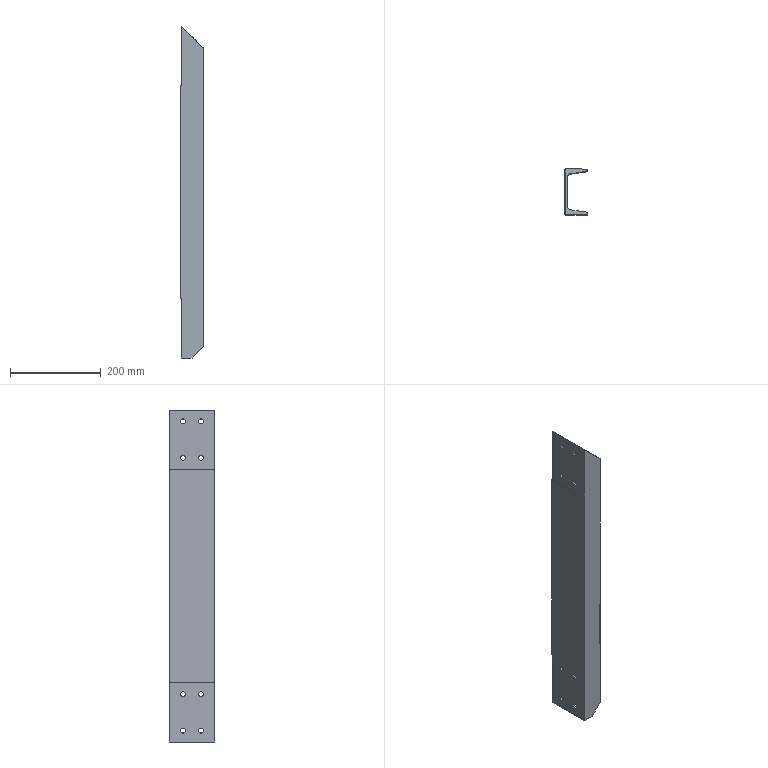Part | SolidWorks | features ICE 3, Extrusion 1, HoleWzd 1 | 1 solid | 40 faces | box 50 x 100 x 730 mm | volume 916470 mm3 | cylinder 24 | plane 16 | commonest cylinder face diameters 11 x16 5 x4 9 x2 17 x2
STEP:
#1=CARTESIAN_POINT('',(20.5,-9.132,10.));
#2=VERTEX_POINT('',#1);
#3=CARTESIAN_POINT('',(20.5,-9.132,15.));
#4=VERTEX_POINT('',#3);
#5=CARTESIAN_POINT('',(20.5,-9.132,10.));
#6=CARTESIAN_POINT('',(15.5,-9.835,10.));
#7=CARTESIAN_POINT('',(15.5,-9.835,15.));
#8=CARTESIAN_POINT('',(20.5,-9.132,15.));
#9=(BOUNDED_CURVE()B_SPLINE_CURVE(3,(#5,#6,#7,#8),.UNSPECIFIED.,.F.,.F.)B_SPLINE_CURVE_WITH_KNOTS((4,4),(1.571,4.712),.UNSPECIFIED.)CURVE()GEOMETRIC_REPRESENTATION_ITEM()RATIONAL_B_SPLINE_CURVE((1.,0.3333,0.3333,1.))REPRESENTATION_ITEM(''));
#10=EDGE_CURVE('',#2,#4,#9,.T.);
#11=ORIENTED_EDGE('',*,*,#10,.F.);
#12=CARTESIAN_POINT('',(20.5,0.,10.));
#13=VERTEX_POINT('',#12);
#14=CARTESIAN_POINT('',(20.5,0.,10.));
#15=DIRECTION('',(0.,1.,0.));
#16=VECTOR('',#15,1000.);
#17=LINE('',#14,#16);
#18=EDGE_CURVE('',#2,#13,#17,.T.);
#19=ORIENTED_EDGE('',*,*,#18,.T.);
#20=CARTESIAN_POINT('',(20.5,0.,15.));
#21=VERTEX_POINT('',#20);
#22=CARTESIAN_POINT('',(20.5,0.,12.5));
#23=DIRECTION('',(0.,1.,0.));
#24=DIRECTION('',(0.,0.,1.));
#25=AXIS2_PLACEMENT_3D('',#22,#23,#24);
#26=CIRCLE('',#25,2.5);
#27=EDGE_CURVE('',#13,#21,#26,.T.);
#28=ORIENTED_EDGE('',*,*,#27,.T.);
#29=CARTESIAN_POINT('',(20.5,0.,15.));
#30=DIRECTION('',(0.,1.,0.));
#31=VECTOR('',#30,1000.);
#32=LINE('',#29,#31);
#33=EDGE_CURVE('',#4,#21,#32,.T.);
#34=ORIENTED_EDGE('',*,*,#33,.F.);
#35=EDGE_LOOP('',(#11,#19,#28,#34));
#36=FACE_OUTER_BOUND('',#35,.T.);
#37=CARTESIAN_POINT('',(20.5,0.,12.5));
#38=DIRECTION('',(0.,1.,0.));
#39=DIRECTION('',(0.,0.,1.));
#40=AXIS2_PLACEMENT_3D('',#37,#38,#39);
#41=CYLINDRICAL_SURFACE('',#40,2.5);
#42=ADVANCED_FACE('',(#36),#41,.F.);
#43=CARTESIAN_POINT('',(20.5,-9.132,130.));
#44=VERTEX_POINT('',#43);
#45=CARTESIAN_POINT('',(20.5,-9.132,135.));
#46=VERTEX_POINT('',#45);
#47=CARTESIAN_POINT('',(20.5,-9.132,130.));
#48=CARTESIAN_POINT('',(15.5,-9.835,130.));
#49=CARTESIAN_POINT('',(15.5,-9.835,135.));
#50=CARTESIAN_POINT('',(20.5,-9.132,135.));
#51=(BOUNDED_CURVE()B_SPLINE_CURVE(3,(#47,#48,#49,#50),.UNSPECIFIED.,.F.,.F.)B_SPLINE_CURVE_WITH_KNOTS((4,4),(1.571,4.712),.UNSPECIFIED.)CURVE()GEOMETRIC_REPRESENTATION_ITEM()RATIONAL_B_SPLINE_CURVE((1.,0.3333,0.3333,1.))REPRESENTATION_ITEM(''));
#52=EDGE_CURVE('',#44,#46,#51,.T.);
#53=ORIENTED_EDGE('',*,*,#52,.F.);
#54=CARTESIAN_POINT('',(20.5,0.,130.));
#55=VERTEX_POINT('',#54);
#56=CARTESIAN_POINT('',(20.5,0.,130.));
#57=DIRECTION('',(0.,1.,0.));
#58=VECTOR('',#57,1000.);
#59=LINE('',#56,#58);
#60=EDGE_CURVE('',#44,#55,#59,.T.);
#61=ORIENTED_EDGE('',*,*,#60,.T.);
#62=CARTESIAN_POINT('',(20.5,0.,135.));
#63=VERTEX_POINT('',#62);
#64=CARTESIAN_POINT('',(20.5,0.,132.5));
#65=DIRECTION('',(0.,1.,0.));
#66=DIRECTION('',(0.,0.,1.));
#67=AXIS2_PLACEMENT_3D('',#64,#65,#66);
#68=CIRCLE('',#67,2.5);
#69=EDGE_CURVE('',#55,#63,#68,.T.);
#70=ORIENTED_EDGE('',*,*,#69,.T.);
#71=CARTESIAN_POINT('',(20.5,0.,135.));
#72=DIRECTION('',(0.,1.,0.));
#73=VECTOR('',#72,1000.);
#74=LINE('',#71,#73);
#75=EDGE_CURVE('',#46,#63,#74,.T.);
#76=ORIENTED_EDGE('',*,*,#75,.F.);
#77=EDGE_LOOP('',(#53,#61,#70,#76));
#78=FACE_OUTER_BOUND('',#77,.T.);
#79=CARTESIAN_POINT('',(20.5,0.,132.5));
#80=DIRECTION('',(0.,1.,0.));
#81=DIRECTION('',(0.,0.,1.));
#82=AXIS2_PLACEMENT_3D('',#79,#80,#81);
#83=CYLINDRICAL_SURFACE('',#82,2.5);
#84=ADVANCED_FACE('',(#78),#83,.F.);
#85=CARTESIAN_POINT('',(6.,-24.5,625.));
#86=VERTEX_POINT('',#85);
#87=CARTESIAN_POINT('',(6.,-35.5,625.));
#88=VERTEX_POINT('',#87);
#89=CARTESIAN_POINT('',(6.,-30.,625.));
#90=DIRECTION('',(-1.,0.,0.));
#91=DIRECTION('',(0.,-1.,0.));
#92=AXIS2_PLACEMENT_3D('',#89,#90,#91);
#93=CIRCLE('',#92,5.5);
#94=EDGE_CURVE('',#86,#88,#93,.T.);
#95=ORIENTED_EDGE('',*,*,#94,.F.);
#96=CARTESIAN_POINT('',(1.,-24.5,625.));
#97=VERTEX_POINT('',#96);
#98=CARTESIAN_POINT('',(11.,-24.5,625.));
#99=DIRECTION('',(-1.,0.,0.));
#100=VECTOR('',#99,1000.);
#101=LINE('',#98,#100);
#102=EDGE_CURVE('',#86,#97,#101,.T.);
#103=ORIENTED_EDGE('',*,*,#102,.T.);
#104=CARTESIAN_POINT('',(1.,-35.5,625.));
#105=VERTEX_POINT('',#104);
#106=CARTESIAN_POINT('',(1.,-30.,625.));
#107=DIRECTION('',(-1.,0.,0.));
#108=DIRECTION('',(0.,1.,0.));
#109=AXIS2_PLACEMENT_3D('',#106,#107,#108);
#110=CIRCLE('',#109,5.5);
#111=EDGE_CURVE('',#97,#105,#110,.T.);
#112=ORIENTED_EDGE('',*,*,#111,.T.);
#113=CARTESIAN_POINT('',(11.,-35.5,625.));
#114=DIRECTION('',(-1.,0.,0.));
#115=VECTOR('',#114,1000.);
#116=LINE('',#113,#115);
#117=EDGE_CURVE('',#88,#105,#116,.T.);
#118=ORIENTED_EDGE('',*,*,#117,.F.);
#119=EDGE_LOOP('',(#95,#103,#112,#118));
#120=FACE_OUTER_BOUND('',#119,.T.);
#121=CARTESIAN_POINT('',(11.,-30.,625.));
#122=DIRECTION('',(-1.,0.,0.));
#123=DIRECTION('',(0.,-1.,0.));
#124=AXIS2_PLACEMENT_3D('',#121,#122,#123);
#125=CYLINDRICAL_SURFACE('',#124,5.5);
#126=ADVANCED_FACE('',(#120),#125,.F.);
#127=CARTESIAN_POINT('',(6.,-64.5,705.));
#128=VERTEX_POINT('',#127);
#129=CARTESIAN_POINT('',(6.,-75.5,705.));
#130=VERTEX_POINT('',#129);
#131=CARTESIAN_POINT('',(6.,-70.,705.));
#132=DIRECTION('',(-1.,0.,0.));
#133=DIRECTION('',(0.,-1.,0.));
#134=AXIS2_PLACEMENT_3D('',#131,#132,#133);
#135=CIRCLE('',#134,5.5);
#136=EDGE_CURVE('',#128,#130,#135,.T.);
#137=ORIENTED_EDGE('',*,*,#136,.F.);
#138=CARTESIAN_POINT('',(1.,-64.5,705.));
#139=VERTEX_POINT('',#138);
#140=CARTESIAN_POINT('',(11.,-64.5,705.));
#141=DIRECTION('',(-1.,0.,0.));
#142=VECTOR('',#141,1000.);
#143=LINE('',#140,#142);
#144=EDGE_CURVE('',#128,#139,#143,.T.);
#145=ORIENTED_EDGE('',*,*,#144,.T.);
#146=CARTESIAN_POINT('',(1.,-75.5,705.));
#147=VERTEX_POINT('',#146);
#148=CARTESIAN_POINT('',(1.,-70.,705.));
#149=DIRECTION('',(-1.,0.,0.));
#150=DIRECTION('',(0.,1.,0.));
#151=AXIS2_PLACEMENT_3D('',#148,#149,#150);
#152=CIRCLE('',#151,5.5);
#153=EDGE_CURVE('',#139,#147,#152,.T.);
#154=ORIENTED_EDGE('',*,*,#153,.T.);
#155=CARTESIAN_POINT('',(11.,-75.5,705.));
#156=DIRECTION('',(-1.,0.,0.));
#157=VECTOR('',#156,1000.);
#158=LINE('',#155,#157);
#159=EDGE_CURVE('',#130,#147,#158,.T.);
#160=ORIENTED_EDGE('',*,*,#159,.F.);
#161=EDGE_LOOP('',(#137,#145,#154,#160));
#162=FACE_OUTER_BOUND('',#161,.T.);
#163=CARTESIAN_POINT('',(11.,-70.,705.));
#164=DIRECTION('',(-1.,0.,0.));
#165=DIRECTION('',(0.,-1.,0.));
#166=AXIS2_PLACEMENT_3D('',#163,#164,#165);
#167=CYLINDRICAL_SURFACE('',#166,5.5);
#168=ADVANCED_FACE('',(#162),#167,.F.);
#169=CARTESIAN_POINT('',(6.,-64.5,625.));
#170=VERTEX_POINT('',#169);
#171=CARTESIAN_POINT('',(6.,-75.5,625.));
#172=VERTEX_POINT('',#171);
#173=CARTESIAN_POINT('',(6.,-70.,625.));
#174=DIRECTION('',(-1.,0.,0.));
#175=DIRECTION('',(0.,-1.,0.));
#176=AXIS2_PLACEMENT_3D('',#173,#174,#175);
#177=CIRCLE('',#176,5.5);
#178=EDGE_CURVE('',#170,#172,#177,.T.);
#179=ORIENTED_EDGE('',*,*,#178,.F.);
#180=CARTESIAN_POINT('',(1.,-64.5,625.));
#181=VERTEX_POINT('',#180);
#182=CARTESIAN_POINT('',(11.,-64.5,625.));
#183=DIRECTION('',(-1.,0.,0.));
#184=VECTOR('',#183,1000.);
#185=LINE('',#182,#184);
#186=EDGE_CURVE('',#170,#181,#185,.T.);
#187=ORIENTED_EDGE('',*,*,#186,.T.);
#188=CARTESIAN_POINT('',(1.,-75.5,625.));
#189=VERTEX_POINT('',#188);
#190=CARTESIAN_POINT('',(1.,-70.,625.));
#191=DIRECTION('',(-1.,0.,0.));
#192=DIRECTION('',(0.,1.,0.));
#193=AXIS2_PLACEMENT_3D('',#190,#191,#192);
#194=CIRCLE('',#193,5.5);
#195=EDGE_CURVE('',#181,#189,#194,.T.);
#196=ORIENTED_EDGE('',*,*,#195,.T.);
#197=CARTESIAN_POINT('',(11.,-75.5,625.));
#198=DIRECTION('',(-1.,0.,0.));
#199=VECTOR('',#198,1000.);
#200=LINE('',#197,#199);
#201=EDGE_CURVE('',#172,#189,#200,.T.);
#202=ORIENTED_EDGE('',*,*,#201,.F.);
#203=EDGE_LOOP('',(#179,#187,#196,#202));
#204=FACE_OUTER_BOUND('',#203,.T.);
#205=CARTESIAN_POINT('',(11.,-70.,625.));
#206=DIRECTION('',(-1.,0.,0.));
#207=DIRECTION('',(0.,-1.,0.));
#208=AXIS2_PLACEMENT_3D('',#205,#206,#207);
#209=CYLINDRICAL_SURFACE('',#208,5.5);
#210=ADVANCED_FACE('',(#204),#209,.F.);
#211=CARTESIAN_POINT('',(6.,-24.5,705.));
#212=VERTEX_POINT('',#211);
#213=CARTESIAN_POINT('',(6.,-35.5,705.));
#214=VERTEX_POINT('',#213);
#215=CARTESIAN_POINT('',(6.,-30.,705.));
#216=DIRECTION('',(-1.,0.,0.));
#217=DIRECTION('',(0.,-1.,0.));
#218=AXIS2_PLACEMENT_3D('',#215,#216,#217);
#219=CIRCLE('',#218,5.5);
#220=EDGE_CURVE('',#212,#214,#219,.T.);
#221=ORIENTED_EDGE('',*,*,#220,.F.);
#222=CARTESIAN_POINT('',(1.,-24.5,705.));
#223=VERTEX_POINT('',#222);
#224=CARTESIAN_POINT('',(11.,-24.5,705.));
#225=DIRECTION('',(-1.,0.,0.));
#226=VECTOR('',#225,1000.);
#227=LINE('',#224,#226);
#228=EDGE_CURVE('',#212,#223,#227,.T.);
#229=ORIENTED_EDGE('',*,*,#228,.T.);
#230=CARTESIAN_POINT('',(1.,-35.5,705.));
#231=VERTEX_POINT('',#230);
#232=CARTESIAN_POINT('',(1.,-30.,705.));
#233=DIRECTION('',(-1.,0.,0.));
#234=DIRECTION('',(0.,1.,0.));
#235=AXIS2_PLACEMENT_3D('',#232,#233,#234);
#236=CIRCLE('',#235,5.5);
#237=EDGE_CURVE('',#223,#231,#236,.T.);
#238=ORIENTED_EDGE('',*,*,#237,.T.);
#239=CARTESIAN_POINT('',(11.,-35.5,705.));
#240=DIRECTION('',(-1.,0.,0.));
#241=VECTOR('',#240,1000.);
#242=LINE('',#239,#241);
#243=EDGE_CURVE('',#214,#231,#242,.T.);
#244=ORIENTED_EDGE('',*,*,#243,.F.);
#245=EDGE_LOOP('',(#221,#229,#238,#244));
#246=FACE_OUTER_BOUND('',#245,.T.);
#247=CARTESIAN_POINT('',(11.,-30.,705.));
#248=DIRECTION('',(-1.,0.,0.));
#249=DIRECTION('',(0.,-1.,0.));
#250=AXIS2_PLACEMENT_3D('',#247,#248,#249);
#251=CYLINDRICAL_SURFACE('',#250,5.5);
#252=ADVANCED_FACE('',(#246),#251,.F.);
#253=CARTESIAN_POINT('',(6.,-64.5,105.));
#254=VERTEX_POINT('',#253);
#255=CARTESIAN_POINT('',(6.,-75.5,105.));
#256=VERTEX_POINT('',#255);
#257=CARTESIAN_POINT('',(6.,-70.,105.));
#258=DIRECTION('',(-1.,0.,0.));
#259=DIRECTION('',(0.,-1.,0.));
#260=AXIS2_PLACEMENT_3D('',#257,#258,#259);
#261=CIRCLE('',#260,5.5);
#262=EDGE_CURVE('',#254,#256,#261,.T.);
#263=ORIENTED_EDGE('',*,*,#262,.F.);
#264=CARTESIAN_POINT('',(1.,-64.5,105.));
#265=VERTEX_POINT('',#264);
#266=CARTESIAN_POINT('',(11.,-64.5,105.));
#267=DIRECTION('',(-1.,0.,0.));
#268=VECTOR('',#267,1000.);
#269=LINE('',#266,#268);
#270=EDGE_CURVE('',#254,#265,#269,.T.);
#271=ORIENTED_EDGE('',*,*,#270,.T.);
#272=CARTESIAN_POINT('',(1.,-75.5,105.));
#273=VERTEX_POINT('',#272);
#274=CARTESIAN_POINT('',(1.,-70.,105.));
#275=DIRECTION('',(-1.,0.,0.));
#276=DIRECTION('',(0.,-1.,0.));
#277=AXIS2_PLACEMENT_3D('',#274,#275,#276);
#278=CIRCLE('',#277,5.5);
#279=EDGE_CURVE('',#265,#273,#278,.T.);
#280=ORIENTED_EDGE('',*,*,#279,.T.);
#281=CARTESIAN_POINT('',(11.,-75.5,105.));
#282=DIRECTION('',(-1.,0.,0.));
#283=VECTOR('',#282,1000.);
#284=LINE('',#281,#283);
#285=EDGE_CURVE('',#256,#273,#284,.T.);
#286=ORIENTED_EDGE('',*,*,#285,.F.);
#287=EDGE_LOOP('',(#263,#271,#280,#286));
#288=FACE_OUTER_BOUND('',#287,.T.);
#289=CARTESIAN_POINT('',(11.,-70.,105.));
#290=DIRECTION('',(-1.,0.,0.));
#291=DIRECTION('',(0.,-1.,0.));
#292=AXIS2_PLACEMENT_3D('',#289,#290,#291);
#293=CYLINDRICAL_SURFACE('',#292,5.5);
#294=ADVANCED_FACE('',(#288),#293,.F.);
#295=CARTESIAN_POINT('',(6.,-64.5,25.));
#296=VERTEX_POINT('',#295);
#297=CARTESIAN_POINT('',(6.,-75.5,25.));
#298=VERTEX_POINT('',#297);
#299=CARTESIAN_POINT('',(6.,-70.,25.));
#300=DIRECTION('',(-1.,0.,0.));
#301=DIRECTION('',(0.,-1.,0.));
#302=AXIS2_PLACEMENT_3D('',#299,#300,#301);
#303=CIRCLE('',#302,5.5);
#304=EDGE_CURVE('',#296,#298,#303,.T.);
#305=ORIENTED_EDGE('',*,*,#304,.F.);
#306=CARTESIAN_POINT('',(1.,-64.5,25.));
#307=VERTEX_POINT('',#306);
#308=CARTESIAN_POINT('',(11.,-64.5,25.));
#309=DIRECTION('',(-1.,0.,0.));
#310=VECTOR('',#309,1000.);
#311=LINE('',#308,#310);
#312=EDGE_CURVE('',#296,#307,#311,.T.);
#313=ORIENTED_EDGE('',*,*,#312,.T.);
#314=CARTESIAN_POINT('',(1.,-75.5,25.));
#315=VERTEX_POINT('',#314);
#316=CARTESIAN_POINT('',(1.,-70.,25.));
#317=DIRECTION('',(-1.,0.,0.));
#318=DIRECTION('',(0.,-1.,0.));
#319=AXIS2_PLACEMENT_3D('',#316,#317,#318);
#320=CIRCLE('',#319,5.5);
#321=EDGE_CURVE('',#307,#315,#320,.T.);
#322=ORIENTED_EDGE('',*,*,#321,.T.);
#323=CARTESIAN_POINT('',(11.,-75.5,25.));
#324=DIRECTION('',(-1.,0.,0.));
#325=VECTOR('',#324,1000.);
#326=LINE('',#323,#325);
#327=EDGE_CURVE('',#298,#315,#326,.T.);
#328=ORIENTED_EDGE('',*,*,#327,.F.);
#329=EDGE_LOOP('',(#305,#313,#322,#328));
#330=FACE_OUTER_BOUND('',#329,.T.);
#331=CARTESIAN_POINT('',(11.,-70.,25.));
#332=DIRECTION('',(-1.,0.,0.));
#333=DIRECTION('',(0.,-1.,0.));
#334=AXIS2_PLACEMENT_3D('',#331,#332,#333);
#335=CYLINDRICAL_SURFACE('',#334,5.5);
#336=ADVANCED_FACE('',(#330),#335,.F.);
#337=CARTESIAN_POINT('',(6.,-24.5,105.));
#338=VERTEX_POINT('',#337);
#339=CARTESIAN_POINT('',(6.,-35.5,105.));
#340=VERTEX_POINT('',#339);
#341=CARTESIAN_POINT('',(6.,-30.,105.));
#342=DIRECTION('',(-1.,0.,0.));
#343=DIRECTION('',(0.,-1.,0.));
#344=AXIS2_PLACEMENT_3D('',#341,#342,#343);
#345=CIRCLE('',#344,5.5);
#346=EDGE_CURVE('',#338,#340,#345,.T.);
#347=ORIENTED_EDGE('',*,*,#346,.F.);
#348=CARTESIAN_POINT('',(1.,-24.5,105.));
#349=VERTEX_POINT('',#348);
#350=CARTESIAN_POINT('',(11.,-24.5,105.));
#351=DIRECTION('',(-1.,0.,0.));
#352=VECTOR('',#351,1000.);
#353=LINE('',#350,#352);
#354=EDGE_CURVE('',#338,#349,#353,.T.);
#355=ORIENTED_EDGE('',*,*,#354,.T.);
#356=CARTESIAN_POINT('',(1.,-35.5,105.));
#357=VERTEX_POINT('',#356);
#358=CARTESIAN_POINT('',(1.,-30.,105.));
#359=DIRECTION('',(-1.,0.,0.));
#360=DIRECTION('',(0.,-1.,0.));
#361=AXIS2_PLACEMENT_3D('',#358,#359,#360);
#362=CIRCLE('',#361,5.5);
#363=EDGE_CURVE('',#349,#357,#362,.T.);
#364=ORIENTED_EDGE('',*,*,#363,.T.);
#365=CARTESIAN_POINT('',(11.,-35.5,105.));
#366=DIRECTION('',(-1.,0.,0.));
#367=VECTOR('',#366,1000.);
#368=LINE('',#365,#367);
#369=EDGE_CURVE('',#340,#357,#368,.T.);
#370=ORIENTED_EDGE('',*,*,#369,.F.);
#371=EDGE_LOOP('',(#347,#355,#364,#370));
#372=FACE_OUTER_BOUND('',#371,.T.);
#373=CARTESIAN_POINT('',(11.,-30.,105.));
#374=DIRECTION('',(-1.,0.,0.));
#375=DIRECTION('',(0.,-1.,0.));
#376=AXIS2_PLACEMENT_3D('',#373,#374,#375);
#377=CYLINDRICAL_SURFACE('',#376,5.5);
#378=ADVANCED_FACE('',(#372),#377,.F.);
#379=CARTESIAN_POINT('',(6.,-24.5,25.));
#380=VERTEX_POINT('',#379);
#381=CARTESIAN_POINT('',(6.,-35.5,25.));
#382=VERTEX_POINT('',#381);
#383=CARTESIAN_POINT('',(6.,-30.,25.));
#384=DIRECTION('',(-1.,0.,0.));
#385=DIRECTION('',(0.,-1.,0.));
#386=AXIS2_PLACEMENT_3D('',#383,#384,#385);
#387=CIRCLE('',#386,5.5);
#388=EDGE_CURVE('',#380,#382,#387,.T.);
#389=ORIENTED_EDGE('',*,*,#388,.F.);
#390=CARTESIAN_POINT('',(1.,-24.5,25.));
#391=VERTEX_POINT('',#390);
#392=CARTESIAN_POINT('',(11.,-24.5,25.));
#393=DIRECTION('',(-1.,0.,0.));
#394=VECTOR('',#393,1000.);
#395=LINE('',#392,#394);
#396=EDGE_CURVE('',#380,#391,#395,.T.);
#397=ORIENTED_EDGE('',*,*,#396,.T.);
#398=CARTESIAN_POINT('',(1.,-35.5,25.));
#399=VERTEX_POINT('',#398);
#400=CARTESIAN_POINT('',(1.,-30.,25.));
#401=DIRECTION('',(-1.,0.,0.));
#402=DIRECTION('',(0.,-1.,0.));
#403=AXIS2_PLACEMENT_3D('',#400,#401,#402);
#404=CIRCLE('',#403,5.5);
#405=EDGE_CURVE('',#391,#399,#404,.T.);
#406=ORIENTED_EDGE('',*,*,#405,.T.);
#407=CARTESIAN_POINT('',(11.,-35.5,25.));
#408=DIRECTION('',(-1.,0.,0.));
#409=VECTOR('',#408,1000.);
#410=LINE('',#407,#409);
#411=EDGE_CURVE('',#382,#399,#410,.T.);
#412=ORIENTED_EDGE('',*,*,#411,.F.);
#413=EDGE_LOOP('',(#389,#397,#406,#412));
#414=FACE_OUTER_BOUND('',#413,.T.);
#415=CARTESIAN_POINT('',(11.,-30.,25.));
#416=DIRECTION('',(-1.,0.,0.));
#417=DIRECTION('',(0.,-1.,0.));
#418=AXIS2_PLACEMENT_3D('',#415,#416,#417);
#419=CYLINDRICAL_SURFACE('',#418,5.5);
#420=ADVANCED_FACE('',(#414),#419,.F.);
#421=CARTESIAN_POINT('',(20.5,0.,12.5));
#422=DIRECTION('',(0.,1.,0.));
#423=DIRECTION('',(0.,0.,1.));
#424=AXIS2_PLACEMENT_3D('',#421,#422,#423);
#425=CIRCLE('',#424,2.5);
#426=EDGE_CURVE('',#21,#13,#425,.T.);
#427=ORIENTED_EDGE('',*,*,#426,.F.);
#428=ORIENTED_EDGE('',*,*,#27,.F.);
#429=EDGE_LOOP('',(#427,#428));
#430=FACE_BOUND('',#429,.T.);
#431=CARTESIAN_POINT('',(20.5,0.,132.5));
#432=DIRECTION('',(0.,1.,0.));
#433=DIRECTION('',(0.,0.,1.));
#434=AXIS2_PLACEMENT_3D('',#431,#432,#433);
#435=CIRCLE('',#434,2.5);
#436=EDGE_CURVE('',#63,#55,#435,.T.);
#437=ORIENTED_EDGE('',*,*,#436,.F.);
#438=ORIENTED_EDGE('',*,*,#69,.F.);
#439=EDGE_LOOP('',(#437,#438));
#440=FACE_BOUND('',#439,.T.);
#441=CARTESIAN_POINT('',(1.,0.,0.));
#442=VERTEX_POINT('',#441);
#443=CARTESIAN_POINT('',(1.,0.,130.));
#444=VERTEX_POINT('',#443);
#445=CARTESIAN_POINT('',(1.,0.,750.));
#446=DIRECTION('',(0.,0.,1.));
#447=VECTOR('',#446,1000.);
#448=LINE('',#445,#447);
#449=EDGE_CURVE('',#442,#444,#448,.T.);
#450=ORIENTED_EDGE('',*,*,#449,.T.);
#451=CARTESIAN_POINT('',(0.,0.,130.));
#452=VERTEX_POINT('',#451);
#453=CARTESIAN_POINT('',(0.,0.,130.));
#454=DIRECTION('',(-1.,0.,0.));
#455=VECTOR('',#454,1000.);
#456=LINE('',#453,#455);
#457=EDGE_CURVE('',#444,#452,#456,.T.);
#458=ORIENTED_EDGE('',*,*,#457,.T.);
#459=CARTESIAN_POINT('',(0.,0.,600.));
#460=VERTEX_POINT('',#459);
#461=CARTESIAN_POINT('',(0.,0.,750.));
#462=DIRECTION('',(0.,0.,-1.));
#463=VECTOR('',#462,1000.);
#464=LINE('',#461,#463);
#465=EDGE_CURVE('',#460,#452,#464,.T.);
#466=ORIENTED_EDGE('',*,*,#465,.F.);
#467=CARTESIAN_POINT('',(1.,0.,600.));
#468=VERTEX_POINT('',#467);
#469=CARTESIAN_POINT('',(0.,0.,600.));
#470=DIRECTION('',(1.,0.,0.));
#471=VECTOR('',#470,1000.);
#472=LINE('',#469,#471);
#473=EDGE_CURVE('',#460,#468,#472,.T.);
#474=ORIENTED_EDGE('',*,*,#473,.T.);
#475=CARTESIAN_POINT('',(1.,0.,730.));
#476=VERTEX_POINT('',#475);
#477=CARTESIAN_POINT('',(1.,0.,750.));
#478=DIRECTION('',(0.,0.,1.));
#479=VECTOR('',#478,1000.);
#480=LINE('',#477,#479);
#481=EDGE_CURVE('',#468,#476,#480,.T.);
#482=ORIENTED_EDGE('',*,*,#481,.T.);
#483=CARTESIAN_POINT('',(50.,0.,681.));
#484=VERTEX_POINT('',#483);
#485=CARTESIAN_POINT('',(258.993,0.,472.007));
#486=DIRECTION('',(-0.7071,0.,0.7071));
#487=VECTOR('',#486,1000.);
#488=LINE('',#485,#487);
#489=EDGE_CURVE('',#484,#476,#488,.T.);
#490=ORIENTED_EDGE('',*,*,#489,.F.);
#491=CARTESIAN_POINT('',(50.,0.,25.));
#492=VERTEX_POINT('',#491);
#493=CARTESIAN_POINT('',(50.,0.,750.));
#494=DIRECTION('',(0.,0.,-1.));
#495=VECTOR('',#494,1000.);
#496=LINE('',#493,#495);
#497=EDGE_CURVE('',#484,#492,#496,.T.);
#498=ORIENTED_EDGE('',*,*,#497,.T.);
#499=CARTESIAN_POINT('',(25.,0.,0.));
#500=VERTEX_POINT('',#499);
#501=CARTESIAN_POINT('',(25.,0.,0.));
#502=DIRECTION('',(0.7071,0.,0.7071));
#503=VECTOR('',#502,1000.);
#504=LINE('',#501,#503);
#505=EDGE_CURVE('',#500,#492,#504,.T.);
#506=ORIENTED_EDGE('',*,*,#505,.F.);
#507=CARTESIAN_POINT('',(0.,0.,0.));
#508=DIRECTION('',(-1.,0.,0.));
#509=VECTOR('',#508,1000.);
#510=LINE('',#507,#509);
#511=EDGE_CURVE('',#500,#442,#510,.T.);
#512=ORIENTED_EDGE('',*,*,#511,.T.);
#513=EDGE_LOOP('',(#450,#458,#466,#474,#482,#490,#498,#506,#512));
#514=FACE_OUTER_BOUND('',#513,.T.);
#515=CARTESIAN_POINT('',(0.,0.,750.));
#516=DIRECTION('',(0.,-1.,0.));
#517=DIRECTION('',(0.,0.,-1.));
#518=AXIS2_PLACEMENT_3D('',#515,#516,#517);
#519=PLANE('',#518);
#520=ADVANCED_FACE('',(#430,#440,#514),#519,.F.);
#521=ORIENTED_EDGE('',*,*,#465,.T.);
#522=CARTESIAN_POINT('',(0.,-100.,130.));
#523=VERTEX_POINT('',#522);
#524=CARTESIAN_POINT('',(0.,38.702,130.));
#525=DIRECTION('',(0.,1.,0.));
#526=VECTOR('',#525,1000.);
#527=LINE('',#524,#526);
#528=EDGE_CURVE('',#523,#452,#527,.T.);
#529=ORIENTED_EDGE('',*,*,#528,.F.);
#530=CARTESIAN_POINT('',(0.,-100.,600.));
#531=VERTEX_POINT('',#530);
#532=CARTESIAN_POINT('',(0.,-100.,750.));
#533=DIRECTION('',(0.,0.,-1.));
#534=VECTOR('',#533,1000.);
#535=LINE('',#532,#534);
#536=EDGE_CURVE('',#531,#523,#535,.T.);
#537=ORIENTED_EDGE('',*,*,#536,.F.);
#538=CARTESIAN_POINT('',(0.,272.776,600.));
#539=DIRECTION('',(0.,-1.,0.));
#540=VECTOR('',#539,1000.);
#541=LINE('',#538,#540);
#542=EDGE_CURVE('',#460,#531,#541,.T.);
#543=ORIENTED_EDGE('',*,*,#542,.F.);
#544=EDGE_LOOP('',(#521,#529,#537,#543));
#545=FACE_OUTER_BOUND('',#544,.T.);
#546=CARTESIAN_POINT('',(0.,0.,750.));
#547=DIRECTION('',(1.,0.,0.));
#548=DIRECTION('',(0.,1.,0.));
#549=AXIS2_PLACEMENT_3D('',#546,#547,#548);
#550=PLANE('',#549);
#551=ADVANCED_FACE('',(#545),#550,.F.);
#552=ORIENTED_EDGE('',*,*,#536,.T.);
#553=CARTESIAN_POINT('',(1.,-100.,130.));
#554=VERTEX_POINT('',#553);
#555=CARTESIAN_POINT('',(0.,-100.,130.));
#556=DIRECTION('',(1.,0.,0.));
#557=VECTOR('',#556,1000.);
#558=LINE('',#555,#557);
#559=EDGE_CURVE('',#523,#554,#558,.T.);
#560=ORIENTED_EDGE('',*,*,#559,.T.);
#561=CARTESIAN_POINT('',(1.,-100.,0.));
#562=VERTEX_POINT('',#561);
#563=CARTESIAN_POINT('',(1.,-100.,750.));
#564=DIRECTION('',(0.,0.,-1.));
#565=VECTOR('',#564,1000.);
#566=LINE('',#563,#565);
#567=EDGE_CURVE('',#554,#562,#566,.T.);
#568=ORIENTED_EDGE('',*,*,#567,.T.);
#569=CARTESIAN_POINT('',(25.,-100.,0.));
#570=VERTEX_POINT('',#569);
#571=CARTESIAN_POINT('',(0.,-100.,0.));
#572=DIRECTION('',(1.,0.,0.));
#573=VECTOR('',#572,1000.);
#574=LINE('',#571,#573);
#575=EDGE_CURVE('',#562,#570,#574,.T.);
#576=ORIENTED_EDGE('',*,*,#575,.T.);
#577=CARTESIAN_POINT('',(50.,-100.,25.));
#578=VERTEX_POINT('',#577);
#579=CARTESIAN_POINT('',(387.5,-100.,362.5));
#580=DIRECTION('',(0.7071,0.,0.7071));
#581=VECTOR('',#580,1000.);
#582=LINE('',#579,#581);
#583=EDGE_CURVE('',#570,#578,#582,.T.);
#584=ORIENTED_EDGE('',*,*,#583,.T.);
#585=CARTESIAN_POINT('',(50.,-100.,681.));
#586=VERTEX_POINT('',#585);
#587=CARTESIAN_POINT('',(50.,-100.,750.));
#588=DIRECTION('',(0.,0.,-1.));
#589=VECTOR('',#588,1000.);
#590=LINE('',#587,#589);
#591=EDGE_CURVE('',#586,#578,#590,.T.);
#592=ORIENTED_EDGE('',*,*,#591,.F.);
#593=CARTESIAN_POINT('',(1.,-100.,730.));
#594=VERTEX_POINT('',#593);
#595=CARTESIAN_POINT('',(-9.5,-100.,740.5));
#596=DIRECTION('',(-0.7071,0.,0.7071));
#597=VECTOR('',#596,1000.);
#598=LINE('',#595,#597);
#599=EDGE_CURVE('',#586,#594,#598,.T.);
#600=ORIENTED_EDGE('',*,*,#599,.T.);
#601=CARTESIAN_POINT('',(1.,-100.,600.));
#602=VERTEX_POINT('',#601);
#603=CARTESIAN_POINT('',(1.,-100.,750.));
#604=DIRECTION('',(0.,0.,-1.));
#605=VECTOR('',#604,1000.);
#606=LINE('',#603,#605);
#607=EDGE_CURVE('',#594,#602,#606,.T.);
#608=ORIENTED_EDGE('',*,*,#607,.T.);
#609=CARTESIAN_POINT('',(0.,-100.,600.));
#610=DIRECTION('',(-1.,0.,0.));
#611=VECTOR('',#610,1000.);
#612=LINE('',#609,#611);
#613=EDGE_CURVE('',#602,#531,#612,.T.);
#614=ORIENTED_EDGE('',*,*,#613,.T.);
#615=EDGE_LOOP('',(#552,#560,#568,#576,#584,#592,#600,#608,#614));
#616=FACE_OUTER_BOUND('',#615,.T.);
#617=CARTESIAN_POINT('',(0.,-100.,750.));
#618=DIRECTION('',(0.,1.,0.));
#619=DIRECTION('',(0.,0.,1.));
#620=AXIS2_PLACEMENT_3D('',#617,#618,#619);
#621=PLANE('',#620);
#622=ADVANCED_FACE('',(#616),#621,.F.);
#623=CARTESIAN_POINT('',(50.,-98.925,681.));
#624=VERTEX_POINT('',#623);
#625=CARTESIAN_POINT('',(50.,-98.925,25.));
#626=VERTEX_POINT('',#625);
#627=CARTESIAN_POINT('',(50.,-98.925,750.));
#628=DIRECTION('',(0.,0.,-1.));
#629=VECTOR('',#628,1000.);
#630=LINE('',#627,#629);
#631=EDGE_CURVE('',#624,#626,#630,.T.);
#632=ORIENTED_EDGE('',*,*,#631,.F.);
#633=CARTESIAN_POINT('',(50.,-100.,681.));
#634=DIRECTION('',(0.,-1.,0.));
#635=VECTOR('',#634,1000.);
#636=LINE('',#633,#635);
#637=EDGE_CURVE('',#624,#586,#636,.T.);
#638=ORIENTED_EDGE('',*,*,#637,.T.);
#639=ORIENTED_EDGE('',*,*,#591,.T.);
#640=CARTESIAN_POINT('',(50.,-730.,25.));
#641=DIRECTION('',(0.,1.,0.));
#642=VECTOR('',#641,1000.);
#643=LINE('',#640,#642);
#644=EDGE_CURVE('',#578,#626,#643,.T.);
#645=ORIENTED_EDGE('',*,*,#644,.T.);
#646=EDGE_LOOP('',(#632,#638,#639,#645));
#647=FACE_OUTER_BOUND('',#646,.T.);
#648=CARTESIAN_POINT('',(50.,-100.,750.));
#649=DIRECTION('',(-1.,0.,0.));
#650=DIRECTION('',(0.,0.,1.));
#651=AXIS2_PLACEMENT_3D('',#648,#649,#650);
#652=PLANE('',#651);
#653=ADVANCED_FACE('',(#647),#652,.F.);
#654=CARTESIAN_POINT('',(46.126,-94.469,684.874));
#655=VERTEX_POINT('',#654);
#656=CARTESIAN_POINT('',(46.126,-94.469,21.126));
#657=VERTEX_POINT('',#656);
#658=CARTESIAN_POINT('',(46.126,-94.469,750.));
#659=DIRECTION('',(0.,0.,-1.));
#660=VECTOR('',#659,1000.);
#661=LINE('',#658,#660);
#662=EDGE_CURVE('',#655,#657,#661,.T.);
#663=ORIENTED_EDGE('',*,*,#662,.F.);
#664=CARTESIAN_POINT('',(46.126,-94.469,684.874));
#665=CARTESIAN_POINT('',(48.456,-94.797,682.544));
#666=CARTESIAN_POINT('',(50.,-96.572,681.));
#667=CARTESIAN_POINT('',(50.,-98.925,681.));
#668=(BOUNDED_CURVE()B_SPLINE_CURVE(3,(#664,#665,#666,#667),.UNSPECIFIED.,.F.,.F.)B_SPLINE_CURVE_WITH_KNOTS((4,4),(4.852,6.283),.UNSPECIFIED.)CURVE()GEOMETRIC_REPRESENTATION_ITEM()RATIONAL_B_SPLINE_CURVE((1.,0.8365,0.8365,1.))REPRESENTATION_ITEM(''));
#669=EDGE_CURVE('',#655,#624,#668,.T.);
#670=ORIENTED_EDGE('',*,*,#669,.T.);
#671=ORIENTED_EDGE('',*,*,#631,.T.);
#672=CARTESIAN_POINT('',(50.,-98.925,25.));
#673=CARTESIAN_POINT('',(50.,-96.572,25.));
#674=CARTESIAN_POINT('',(48.456,-94.797,23.456));
#675=CARTESIAN_POINT('',(46.126,-94.469,21.126));
#676=(BOUNDED_CURVE()B_SPLINE_CURVE(3,(#672,#673,#674,#675),.UNSPECIFIED.,.F.,.T.)B_SPLINE_CURVE_WITH_KNOTS((4,4),(3.142,4.573),.UNSPECIFIED.)CURVE()GEOMETRIC_REPRESENTATION_ITEM()RATIONAL_B_SPLINE_CURVE((1.,0.8365,0.8365,1.))REPRESENTATION_ITEM(''));
#677=EDGE_CURVE('',#626,#657,#676,.T.);
#678=ORIENTED_EDGE('',*,*,#677,.T.);
#679=EDGE_LOOP('',(#663,#670,#671,#678));
#680=FACE_OUTER_BOUND('',#679,.T.);
#681=CARTESIAN_POINT('',(45.5,-98.925,750.));
#682=DIRECTION('',(0.,0.,-1.));
#683=DIRECTION('',(-1.,0.,0.));
#684=AXIS2_PLACEMENT_3D('',#681,#682,#683);
#685=CYLINDRICAL_SURFACE('',#684,4.5);
#686=ADVANCED_FACE('',(#680),#685,.T.);
#687=CARTESIAN_POINT('',(13.317,-89.858,717.683));
#688=VERTEX_POINT('',#687);
#689=CARTESIAN_POINT('',(13.317,-89.858,0.));
#690=VERTEX_POINT('',#689);
#691=CARTESIAN_POINT('',(13.317,-89.858,750.));
#692=DIRECTION('',(0.,0.,-1.));
#693=VECTOR('',#692,1000.);
#694=LINE('',#691,#693);
#695=EDGE_CURVE('',#688,#690,#694,.T.);
#696=ORIENTED_EDGE('',*,*,#695,.F.);
#697=CARTESIAN_POINT('',(-2.683,-87.609,733.683));
#698=DIRECTION('',(0.7036,-0.09889,-0.7036));
#699=VECTOR('',#698,1000.);
#700=LINE('',#697,#699);
#701=EDGE_CURVE('',#688,#655,#700,.T.);
#702=ORIENTED_EDGE('',*,*,#701,.T.);
#703=ORIENTED_EDGE('',*,*,#662,.T.);
#704=CARTESIAN_POINT('',(25.,-91.5,0.));
#705=VERTEX_POINT('',#704);
#706=CARTESIAN_POINT('',(390.434,-142.858,365.434));
#707=DIRECTION('',(-0.7036,0.09889,-0.7036));
#708=VECTOR('',#707,1000.);
#709=LINE('',#706,#708);
#710=EDGE_CURVE('',#657,#705,#709,.T.);
#711=ORIENTED_EDGE('',*,*,#710,.T.);
#712=CARTESIAN_POINT('',(13.317,-89.858,0.));
#713=DIRECTION('',(-0.9903,0.1392,0.));
#714=VECTOR('',#713,1000.);
#715=LINE('',#712,#714);
#716=EDGE_CURVE('',#705,#690,#715,.T.);
#717=ORIENTED_EDGE('',*,*,#716,.T.);
#718=EDGE_LOOP('',(#696,#702,#703,#711,#717));
#719=FACE_OUTER_BOUND('',#718,.T.);
#720=CARTESIAN_POINT('',(13.317,-89.858,750.));
#721=DIRECTION('',(-0.1392,-0.9903,0.));
#722=DIRECTION('',(0.9903,-0.1392,0.));
#723=AXIS2_PLACEMENT_3D('',#720,#721,#722);
#724=PLANE('',#723);
#725=ADVANCED_FACE('',(#719),#724,.F.);
#726=CARTESIAN_POINT('',(6.,-81.441,725.));
#727=VERTEX_POINT('',#726);
#728=CARTESIAN_POINT('',(6.,-81.441,0.));
#729=VERTEX_POINT('',#728);
#730=CARTESIAN_POINT('',(6.,-81.441,750.));
#731=DIRECTION('',(0.,0.,-1.));
#732=VECTOR('',#731,1000.);
#733=LINE('',#730,#732);
#734=EDGE_CURVE('',#727,#729,#733,.T.);
#735=ORIENTED_EDGE('',*,*,#734,.F.);
#736=CARTESIAN_POINT('',(6.,-81.441,725.));
#737=CARTESIAN_POINT('',(6.,-85.885,725.));
#738=CARTESIAN_POINT('',(8.916,-89.24,722.084));
#739=CARTESIAN_POINT('',(13.317,-89.858,717.683));
#740=(BOUNDED_CURVE()B_SPLINE_CURVE(3,(#736,#737,#738,#739),.UNSPECIFIED.,.F.,.F.)B_SPLINE_CURVE_WITH_KNOTS((4,4),(3.142,4.573),.UNSPECIFIED.)CURVE()GEOMETRIC_REPRESENTATION_ITEM()RATIONAL_B_SPLINE_CURVE((1.,0.8365,0.8365,1.))REPRESENTATION_ITEM(''));
#741=EDGE_CURVE('',#727,#688,#740,.T.);
#742=ORIENTED_EDGE('',*,*,#741,.T.);
#743=ORIENTED_EDGE('',*,*,#695,.T.);
#744=CARTESIAN_POINT('',(14.5,-81.441,0.));
#745=DIRECTION('',(0.,0.,-1.));
#746=DIRECTION('',(1.,0.,0.));
#747=AXIS2_PLACEMENT_3D('',#744,#745,#746);
#748=CIRCLE('',#747,8.5);
#749=EDGE_CURVE('',#690,#729,#748,.T.);
#750=ORIENTED_EDGE('',*,*,#749,.T.);
#751=EDGE_LOOP('',(#735,#742,#743,#750));
#752=FACE_OUTER_BOUND('',#751,.T.);
#753=CARTESIAN_POINT('',(14.5,-81.441,750.));
#754=DIRECTION('',(0.,0.,-1.));
#755=DIRECTION('',(-1.,0.,0.));
#756=AXIS2_PLACEMENT_3D('',#753,#754,#755);
#757=CYLINDRICAL_SURFACE('',#756,8.5);
#758=ADVANCED_FACE('',(#752),#757,.F.);
#759=CARTESIAN_POINT('',(6.,-30.,625.));
#760=DIRECTION('',(-1.,0.,0.));
#761=DIRECTION('',(0.,-1.,0.));
#762=AXIS2_PLACEMENT_3D('',#759,#760,#761);
#763=CIRCLE('',#762,5.5);
#764=EDGE_CURVE('',#88,#86,#763,.T.);
#765=ORIENTED_EDGE('',*,*,#764,.T.);
#766=ORIENTED_EDGE('',*,*,#94,.T.);
#767=EDGE_LOOP('',(#765,#766));
#768=FACE_BOUND('',#767,.T.);
#769=CARTESIAN_POINT('',(6.,-70.,105.));
#770=DIRECTION('',(-1.,0.,0.));
#771=DIRECTION('',(0.,-1.,0.));
#772=AXIS2_PLACEMENT_3D('',#769,#770,#771);
#773=CIRCLE('',#772,5.5);
#774=EDGE_CURVE('',#256,#254,#773,.T.);
#775=ORIENTED_EDGE('',*,*,#774,.T.);
#776=ORIENTED_EDGE('',*,*,#262,.T.);
#777=EDGE_LOOP('',(#775,#776));
#778=FACE_BOUND('',#777,.T.);
#779=CARTESIAN_POINT('',(6.,-70.,25.));
#780=DIRECTION('',(-1.,0.,0.));
#781=DIRECTION('',(0.,-1.,0.));
#782=AXIS2_PLACEMENT_3D('',#779,#780,#781);
#783=CIRCLE('',#782,5.5);
#784=EDGE_CURVE('',#298,#296,#783,.T.);
#785=ORIENTED_EDGE('',*,*,#784,.T.);
#786=ORIENTED_EDGE('',*,*,#304,.T.);
#787=EDGE_LOOP('',(#785,#786));
#788=FACE_BOUND('',#787,.T.);
#789=CARTESIAN_POINT('',(6.,-30.,105.));
#790=DIRECTION('',(-1.,0.,0.));
#791=DIRECTION('',(0.,-1.,0.));
#792=AXIS2_PLACEMENT_3D('',#789,#790,#791);
#793=CIRCLE('',#792,5.5);
#794=EDGE_CURVE('',#340,#338,#793,.T.);
#795=ORIENTED_EDGE('',*,*,#794,.T.);
#796=ORIENTED_EDGE('',*,*,#346,.T.);
#797=EDGE_LOOP('',(#795,#796));
#798=FACE_BOUND('',#797,.T.);
#799=CARTESIAN_POINT('',(6.,-70.,705.));
#800=DIRECTION('',(-1.,0.,0.));
#801=DIRECTION('',(0.,-1.,0.));
#802=AXIS2_PLACEMENT_3D('',#799,#800,#801);
#803=CIRCLE('',#802,5.5);
#804=EDGE_CURVE('',#130,#128,#803,.T.);
#805=ORIENTED_EDGE('',*,*,#804,.T.);
#806=ORIENTED_EDGE('',*,*,#136,.T.);
#807=EDGE_LOOP('',(#805,#806));
#808=FACE_BOUND('',#807,.T.);
#809=CARTESIAN_POINT('',(6.,-70.,625.));
#810=DIRECTION('',(-1.,0.,0.));
#811=DIRECTION('',(0.,-1.,0.));
#812=AXIS2_PLACEMENT_3D('',#809,#810,#811);
#813=CIRCLE('',#812,5.5);
#814=EDGE_CURVE('',#172,#170,#813,.T.);
#815=ORIENTED_EDGE('',*,*,#814,.T.);
#816=ORIENTED_EDGE('',*,*,#178,.T.);
#817=EDGE_LOOP('',(#815,#816));
#818=FACE_BOUND('',#817,.T.);
#819=CARTESIAN_POINT('',(6.,-30.,705.));
#820=DIRECTION('',(-1.,0.,0.));
#821=DIRECTION('',(0.,-1.,0.));
#822=AXIS2_PLACEMENT_3D('',#819,#820,#821);
#823=CIRCLE('',#822,5.5);
#824=EDGE_CURVE('',#214,#212,#823,.T.);
#825=ORIENTED_EDGE('',*,*,#824,.T.);
#826=ORIENTED_EDGE('',*,*,#220,.T.);
#827=EDGE_LOOP('',(#825,#826));
#828=FACE_BOUND('',#827,.T.);
#829=CARTESIAN_POINT('',(6.,-30.,25.));
#830=DIRECTION('',(-1.,0.,0.));
#831=DIRECTION('',(0.,-1.,0.));
#832=AXIS2_PLACEMENT_3D('',#829,#830,#831);
#833=CIRCLE('',#832,5.5);
#834=EDGE_CURVE('',#382,#380,#833,.T.);
#835=ORIENTED_EDGE('',*,*,#834,.T.);
#836=ORIENTED_EDGE('',*,*,#388,.T.);
#837=EDGE_LOOP('',(#835,#836));
#838=FACE_BOUND('',#837,.T.);
#839=CARTESIAN_POINT('',(6.,-18.559,725.));
#840=VERTEX_POINT('',#839);
#841=CARTESIAN_POINT('',(6.,-18.559,0.));
#842=VERTEX_POINT('',#841);
#843=CARTESIAN_POINT('',(6.,-18.559,750.));
#844=DIRECTION('',(0.,0.,-1.));
#845=VECTOR('',#844,1000.);
#846=LINE('',#843,#845);
#847=EDGE_CURVE('',#840,#842,#846,.T.);
#848=ORIENTED_EDGE('',*,*,#847,.F.);
#849=CARTESIAN_POINT('',(6.,-18.559,725.));
#850=DIRECTION('',(0.,-1.,0.));
#851=VECTOR('',#850,1000.);
#852=LINE('',#849,#851);
#853=EDGE_CURVE('',#840,#727,#852,.T.);
#854=ORIENTED_EDGE('',*,*,#853,.T.);
#855=ORIENTED_EDGE('',*,*,#734,.T.);
#856=CARTESIAN_POINT('',(6.,-18.559,0.));
#857=DIRECTION('',(0.,1.,0.));
#858=VECTOR('',#857,1000.);
#859=LINE('',#856,#858);
#860=EDGE_CURVE('',#729,#842,#859,.T.);
#861=ORIENTED_EDGE('',*,*,#860,.T.);
#862=EDGE_LOOP('',(#848,#854,#855,#861));
#863=FACE_OUTER_BOUND('',#862,.T.);
#864=CARTESIAN_POINT('',(6.,-18.559,750.));
#865=DIRECTION('',(-1.,0.,0.));
#866=DIRECTION('',(0.,-1.,0.));
#867=AXIS2_PLACEMENT_3D('',#864,#865,#866);
#868=PLANE('',#867);
#869=ADVANCED_FACE('',(#768,#778,#788,#798,#808,#818,#828,#838,#863),#868,.F.);
#870=CARTESIAN_POINT('',(13.317,-10.142,717.683));
#871=VERTEX_POINT('',#870);
#872=CARTESIAN_POINT('',(13.317,-10.142,0.));
#873=VERTEX_POINT('',#872);
#874=CARTESIAN_POINT('',(13.317,-10.142,750.));
#875=DIRECTION('',(0.,0.,-1.));
#876=VECTOR('',#875,1000.);
#877=LINE('',#874,#876);
#878=EDGE_CURVE('',#871,#873,#877,.T.);
#879=ORIENTED_EDGE('',*,*,#878,.F.);
#880=CARTESIAN_POINT('',(13.317,-10.142,717.683));
#881=CARTESIAN_POINT('',(8.916,-10.76,722.084));
#882=CARTESIAN_POINT('',(6.,-14.115,725.));
#883=CARTESIAN_POINT('',(6.,-18.559,725.));
#884=(BOUNDED_CURVE()B_SPLINE_CURVE(3,(#880,#881,#882,#883),.UNSPECIFIED.,.F.,.F.)B_SPLINE_CURVE_WITH_KNOTS((4,4),(1.71,3.142),.UNSPECIFIED.)CURVE()GEOMETRIC_REPRESENTATION_ITEM()RATIONAL_B_SPLINE_CURVE((1.,0.8365,0.8365,1.))REPRESENTATION_ITEM(''));
#885=EDGE_CURVE('',#871,#840,#884,.T.);
#886=ORIENTED_EDGE('',*,*,#885,.T.);
#887=ORIENTED_EDGE('',*,*,#847,.T.);
#888=CARTESIAN_POINT('',(14.5,-18.559,0.));
#889=DIRECTION('',(0.,0.,-1.));
#890=DIRECTION('',(1.,0.,0.));
#891=AXIS2_PLACEMENT_3D('',#888,#889,#890);
#892=CIRCLE('',#891,8.5);
#893=EDGE_CURVE('',#842,#873,#892,.T.);
#894=ORIENTED_EDGE('',*,*,#893,.T.);
#895=EDGE_LOOP('',(#879,#886,#887,#894));
#896=FACE_OUTER_BOUND('',#895,.T.);
#897=CARTESIAN_POINT('',(14.5,-18.559,750.));
#898=DIRECTION('',(0.,0.,-1.));
#899=DIRECTION('',(-1.,0.,0.));
#900=AXIS2_PLACEMENT_3D('',#897,#898,#899);
#901=CYLINDRICAL_SURFACE('',#900,8.5);
#902=ADVANCED_FACE('',(#896),#901,.F.);
#903=CARTESIAN_POINT('',(20.5,-9.132,15.));
#904=CARTESIAN_POINT('',(25.5,-8.43,15.));
#905=CARTESIAN_POINT('',(25.5,-8.43,10.));
#906=CARTESIAN_POINT('',(20.5,-9.132,10.));
#907=(BOUNDED_CURVE()B_SPLINE_CURVE(3,(#903,#904,#905,#906),.UNSPECIFIED.,.F.,.T.)B_SPLINE_CURVE_WITH_KNOTS((4,4),(4.712,7.854),.UNSPECIFIED.)CURVE()GEOMETRIC_REPRESENTATION_ITEM()RATIONAL_B_SPLINE_CURVE((1.,0.3333,0.3333,1.))REPRESENTATION_ITEM(''));
#908=EDGE_CURVE('',#4,#2,#907,.T.);
#909=ORIENTED_EDGE('',*,*,#908,.T.);
#910=ORIENTED_EDGE('',*,*,#10,.T.);
#911=EDGE_LOOP('',(#909,#910));
#912=FACE_BOUND('',#911,.T.);
#913=CARTESIAN_POINT('',(20.5,-9.132,135.));
#914=CARTESIAN_POINT('',(25.5,-8.43,135.));
#915=CARTESIAN_POINT('',(25.5,-8.43,130.));
#916=CARTESIAN_POINT('',(20.5,-9.132,130.));
#917=(BOUNDED_CURVE()B_SPLINE_CURVE(3,(#913,#914,#915,#916),.UNSPECIFIED.,.F.,.F.)B_SPLINE_CURVE_WITH_KNOTS((4,4),(4.712,7.854),.UNSPECIFIED.)CURVE()GEOMETRIC_REPRESENTATION_ITEM()RATIONAL_B_SPLINE_CURVE((1.,0.3333,0.3333,1.))REPRESENTATION_ITEM(''));
#918=EDGE_CURVE('',#46,#44,#917,.T.);
#919=ORIENTED_EDGE('',*,*,#918,.T.);
#920=ORIENTED_EDGE('',*,*,#52,.T.);
#921=EDGE_LOOP('',(#919,#920));
#922=FACE_BOUND('',#921,.T.);
#923=CARTESIAN_POINT('',(46.126,-5.531,684.874));
#924=VERTEX_POINT('',#923);
#925=CARTESIAN_POINT('',(46.126,-5.531,21.126));
#926=VERTEX_POINT('',#925);
#927=CARTESIAN_POINT('',(46.126,-5.531,750.));
#928=DIRECTION('',(0.,0.,-1.));
#929=VECTOR('',#928,1000.);
#930=LINE('',#927,#929);
#931=EDGE_CURVE('',#924,#926,#930,.T.);
#932=ORIENTED_EDGE('',*,*,#931,.F.);
#933=CARTESIAN_POINT('',(13.882,-10.063,717.118));
#934=DIRECTION('',(-0.7036,-0.09889,0.7036));
#935=VECTOR('',#934,1000.);
#936=LINE('',#933,#935);
#937=EDGE_CURVE('',#924,#871,#936,.T.);
#938=ORIENTED_EDGE('',*,*,#937,.T.);
#939=ORIENTED_EDGE('',*,*,#878,.T.);
#940=CARTESIAN_POINT('',(25.,-8.5,0.));
#941=VERTEX_POINT('',#940);
#942=CARTESIAN_POINT('',(46.126,-5.531,0.));
#943=DIRECTION('',(0.9903,0.1392,0.));
#944=VECTOR('',#943,1000.);
#945=LINE('',#942,#944);
#946=EDGE_CURVE('',#873,#941,#945,.T.);
#947=ORIENTED_EDGE('',*,*,#946,.T.);
#948=CARTESIAN_POINT('',(406.999,45.186,381.999));
#949=DIRECTION('',(0.7036,0.09889,0.7036));
#950=VECTOR('',#949,1000.);
#951=LINE('',#948,#950);
#952=EDGE_CURVE('',#941,#926,#951,.T.);
#953=ORIENTED_EDGE('',*,*,#952,.T.);
#954=EDGE_LOOP('',(#932,#938,#939,#947,#953));
#955=FACE_OUTER_BOUND('',#954,.T.);
#956=CARTESIAN_POINT('',(46.126,-5.531,750.));
#957=DIRECTION('',(-0.1392,0.9903,0.));
#958=DIRECTION('',(-0.9903,-0.1392,0.));
#959=AXIS2_PLACEMENT_3D('',#956,#957,#958);
#960=PLANE('',#959);
#961=ADVANCED_FACE('',(#912,#922,#955),#960,.F.);
#962=CARTESIAN_POINT('',(50.,-1.075,681.));
#963=VERTEX_POINT('',#962);
#964=CARTESIAN_POINT('',(50.,-1.075,25.));
#965=VERTEX_POINT('',#964);
#966=CARTESIAN_POINT('',(50.,-1.075,750.));
#967=DIRECTION('',(0.,0.,-1.));
#968=VECTOR('',#967,1000.);
#969=LINE('',#966,#968);
#970=EDGE_CURVE('',#963,#965,#969,.T.);
#971=ORIENTED_EDGE('',*,*,#970,.F.);
#972=CARTESIAN_POINT('',(50.,-1.075,681.));
#973=CARTESIAN_POINT('',(50.,-3.428,681.));
#974=CARTESIAN_POINT('',(48.456,-5.203,682.544));
#975=CARTESIAN_POINT('',(46.126,-5.531,684.874));
#976=(BOUNDED_CURVE()B_SPLINE_CURVE(3,(#972,#973,#974,#975),.UNSPECIFIED.,.F.,.F.)B_SPLINE_CURVE_WITH_KNOTS((4,4),(0.,1.431),.UNSPECIFIED.)CURVE()GEOMETRIC_REPRESENTATION_ITEM()RATIONAL_B_SPLINE_CURVE((1.,0.8365,0.8365,1.))REPRESENTATION_ITEM(''));
#977=EDGE_CURVE('',#963,#924,#976,.T.);
#978=ORIENTED_EDGE('',*,*,#977,.T.);
#979=ORIENTED_EDGE('',*,*,#931,.T.);
#980=CARTESIAN_POINT('',(46.126,-5.531,21.126));
#981=CARTESIAN_POINT('',(48.456,-5.203,23.456));
#982=CARTESIAN_POINT('',(50.,-3.428,25.));
#983=CARTESIAN_POINT('',(50.,-1.075,25.));
#984=(BOUNDED_CURVE()B_SPLINE_CURVE(3,(#980,#981,#982,#983),.UNSPECIFIED.,.F.,.F.)B_SPLINE_CURVE_WITH_KNOTS((4,4),(1.71,3.142),.UNSPECIFIED.)CURVE()GEOMETRIC_REPRESENTATION_ITEM()RATIONAL_B_SPLINE_CURVE((1.,0.8365,0.8365,1.))REPRESENTATION_ITEM(''));
#985=EDGE_CURVE('',#926,#965,#984,.T.);
#986=ORIENTED_EDGE('',*,*,#985,.T.);
#987=EDGE_LOOP('',(#971,#978,#979,#986));
#988=FACE_OUTER_BOUND('',#987,.T.);
#989=CARTESIAN_POINT('',(45.5,-1.075,750.));
#990=DIRECTION('',(0.,0.,-1.));
#991=DIRECTION('',(-1.,0.,0.));
#992=AXIS2_PLACEMENT_3D('',#989,#990,#991);
#993=CYLINDRICAL_SURFACE('',#992,4.5);
#994=ADVANCED_FACE('',(#988),#993,.T.);
#995=ORIENTED_EDGE('',*,*,#497,.F.);
#996=CARTESIAN_POINT('',(50.,0.,681.));
#997=DIRECTION('',(0.,-1.,0.));
#998=VECTOR('',#997,1000.);
#999=LINE('',#996,#998);
#1000=EDGE_CURVE('',#484,#963,#999,.T.);
#1001=ORIENTED_EDGE('',*,*,#1000,.T.);
#1002=ORIENTED_EDGE('',*,*,#970,.T.);
#1003=CARTESIAN_POINT('',(50.,-730.,25.));
#1004=DIRECTION('',(0.,1.,0.));
#1005=VECTOR('',#1004,1000.);
#1006=LINE('',#1003,#1005);
#1007=EDGE_CURVE('',#965,#492,#1006,.T.);
#1008=ORIENTED_EDGE('',*,*,#1007,.T.);
#1009=EDGE_LOOP('',(#995,#1001,#1002,#1008));
#1010=FACE_OUTER_BOUND('',#1009,.T.);
#1011=CARTESIAN_POINT('',(50.,0.,750.));
#1012=DIRECTION('',(-1.,0.,0.));
#1013=DIRECTION('',(0.,0.,1.));
#1014=AXIS2_PLACEMENT_3D('',#1011,#1012,#1013);
#1015=PLANE('',#1014);
#1016=ADVANCED_FACE('',(#1010),#1015,.F.);
#1017=CARTESIAN_POINT('',(1.,-1.075,0.));
#1018=DIRECTION('',(0.,-1.,0.));
#1019=VECTOR('',#1018,1000.);
#1020=LINE('',#1017,#1019);
#1021=EDGE_CURVE('',#442,#562,#1020,.T.);
#1022=ORIENTED_EDGE('',*,*,#1021,.F.);
#1023=ORIENTED_EDGE('',*,*,#511,.F.);
#1024=CARTESIAN_POINT('',(25.,-1.075,0.));
#1025=DIRECTION('',(0.,1.,0.));
#1026=VECTOR('',#1025,1000.);
#1027=LINE('',#1024,#1026);
#1028=EDGE_CURVE('',#941,#500,#1027,.T.);
#1029=ORIENTED_EDGE('',*,*,#1028,.F.);
#1030=ORIENTED_EDGE('',*,*,#946,.F.);
#1031=ORIENTED_EDGE('',*,*,#893,.F.);
#1032=ORIENTED_EDGE('',*,*,#860,.F.);
#1033=ORIENTED_EDGE('',*,*,#749,.F.);
#1034=ORIENTED_EDGE('',*,*,#716,.F.);
#1035=CARTESIAN_POINT('',(25.,-1.075,0.));
#1036=DIRECTION('',(0.,1.,0.));
#1037=VECTOR('',#1036,1000.);
#1038=LINE('',#1035,#1037);
#1039=EDGE_CURVE('',#570,#705,#1038,.T.);
#1040=ORIENTED_EDGE('',*,*,#1039,.F.);
#1041=ORIENTED_EDGE('',*,*,#575,.F.);
#1042=EDGE_LOOP('',(#1022,#1023,#1029,#1030,#1031,#1032,#1033,#1034,#1040,#1041));
#1043=FACE_OUTER_BOUND('',#1042,.T.);
#1044=CARTESIAN_POINT('',(45.5,-1.075,0.));
#1045=DIRECTION('',(0.,0.,-1.));
#1046=DIRECTION('',(-1.,0.,0.));
#1047=AXIS2_PLACEMENT_3D('',#1044,#1045,#1046);
#1048=PLANE('',#1047);
#1049=ADVANCED_FACE('',(#1043),#1048,.T.);
#1050=ORIENTED_EDGE('',*,*,#1028,.T.);
#1051=ORIENTED_EDGE('',*,*,#505,.T.);
#1052=ORIENTED_EDGE('',*,*,#1007,.F.);
#1053=ORIENTED_EDGE('',*,*,#985,.F.);
#1054=ORIENTED_EDGE('',*,*,#952,.F.);
#1055=EDGE_LOOP('',(#1050,#1051,#1052,#1053,#1054));
#1056=FACE_OUTER_BOUND('',#1055,.T.);
#1057=CARTESIAN_POINT('',(25.,-730.,0.));
#1058=DIRECTION('',(-0.7071,0.,0.7071));
#1059=DIRECTION('',(0.7071,0.,0.7071));
#1060=AXIS2_PLACEMENT_3D('',#1057,#1058,#1059);
#1061=PLANE('',#1060);
#1062=ADVANCED_FACE('',(#1056),#1061,.F.);
#1063=ORIENTED_EDGE('',*,*,#1039,.T.);
#1064=ORIENTED_EDGE('',*,*,#710,.F.);
#1065=ORIENTED_EDGE('',*,*,#677,.F.);
#1066=ORIENTED_EDGE('',*,*,#644,.F.);
#1067=ORIENTED_EDGE('',*,*,#583,.F.);
#1068=EDGE_LOOP('',(#1063,#1064,#1065,#1066,#1067));
#1069=FACE_OUTER_BOUND('',#1068,.T.);
#1070=CARTESIAN_POINT('',(25.,-730.,0.));
#1071=DIRECTION('',(-0.7071,0.,0.7071));
#1072=DIRECTION('',(0.7071,0.,0.7071));
#1073=AXIS2_PLACEMENT_3D('',#1070,#1071,#1072);
#1074=PLANE('',#1073);
#1075=ADVANCED_FACE('',(#1069),#1074,.F.);
#1076=ORIENTED_EDGE('',*,*,#489,.T.);
#1077=CARTESIAN_POINT('',(1.,-730.,730.));
#1078=DIRECTION('',(0.,-1.,0.));
#1079=VECTOR('',#1078,1000.);
#1080=LINE('',#1077,#1079);
#1081=EDGE_CURVE('',#476,#594,#1080,.T.);
#1082=ORIENTED_EDGE('',*,*,#1081,.T.);
#1083=ORIENTED_EDGE('',*,*,#599,.F.);
#1084=ORIENTED_EDGE('',*,*,#637,.F.);
#1085=ORIENTED_EDGE('',*,*,#669,.F.);
#1086=ORIENTED_EDGE('',*,*,#701,.F.);
#1087=ORIENTED_EDGE('',*,*,#741,.F.);
#1088=ORIENTED_EDGE('',*,*,#853,.F.);
#1089=ORIENTED_EDGE('',*,*,#885,.F.);
#1090=ORIENTED_EDGE('',*,*,#937,.F.);
#1091=ORIENTED_EDGE('',*,*,#977,.F.);
#1092=ORIENTED_EDGE('',*,*,#1000,.F.);
#1093=EDGE_LOOP('',(#1076,#1082,#1083,#1084,#1085,#1086,#1087,#1088,#1089,#1090,#1091,#1092));
#1094=FACE_OUTER_BOUND('',#1093,.T.);
#1095=CARTESIAN_POINT('',(258.993,-730.,472.007));
#1096=DIRECTION('',(-0.7071,0.,-0.7071));
#1097=DIRECTION('',(-0.7071,0.,0.7071));
#1098=AXIS2_PLACEMENT_3D('',#1095,#1096,#1097);
#1099=PLANE('',#1098);
#1100=ADVANCED_FACE('',(#1094),#1099,.F.);
#1101=ORIENTED_EDGE('',*,*,#542,.T.);
#1102=ORIENTED_EDGE('',*,*,#613,.F.);
#1103=CARTESIAN_POINT('',(1.,272.776,600.));
#1104=DIRECTION('',(0.,-1.,0.));
#1105=VECTOR('',#1104,1000.);
#1106=LINE('',#1103,#1105);
#1107=EDGE_CURVE('',#468,#602,#1106,.T.);
#1108=ORIENTED_EDGE('',*,*,#1107,.F.);
#1109=ORIENTED_EDGE('',*,*,#473,.F.);
#1110=EDGE_LOOP('',(#1101,#1102,#1108,#1109));
#1111=FACE_OUTER_BOUND('',#1110,.T.);
#1112=CARTESIAN_POINT('',(1.,272.776,600.));
#1113=DIRECTION('',(0.,0.,-1.));
#1114=DIRECTION('',(0.,1.,0.));
#1115=AXIS2_PLACEMENT_3D('',#1112,#1113,#1114);
#1116=PLANE('',#1115);
#1117=ADVANCED_FACE('',(#1111),#1116,.F.);
#1118=CARTESIAN_POINT('',(1.,-30.,625.));
#1119=DIRECTION('',(-1.,0.,0.));
#1120=DIRECTION('',(0.,1.,0.));
#1121=AXIS2_PLACEMENT_3D('',#1118,#1119,#1120);
#1122=CIRCLE('',#1121,5.5);
#1123=EDGE_CURVE('',#105,#97,#1122,.T.);
#1124=ORIENTED_EDGE('',*,*,#1123,.F.);
#1125=ORIENTED_EDGE('',*,*,#111,.F.);
#1126=EDGE_LOOP('',(#1124,#1125));
#1127=FACE_BOUND('',#1126,.T.);
#1128=CARTESIAN_POINT('',(1.,-70.,705.));
#1129=DIRECTION('',(-1.,0.,0.));
#1130=DIRECTION('',(0.,1.,0.));
#1131=AXIS2_PLACEMENT_3D('',#1128,#1129,#1130);
#1132=CIRCLE('',#1131,5.5);
#1133=EDGE_CURVE('',#147,#139,#1132,.T.);
#1134=ORIENTED_EDGE('',*,*,#1133,.F.);
#1135=ORIENTED_EDGE('',*,*,#153,.F.);
#1136=EDGE_LOOP('',(#1134,#1135));
#1137=FACE_BOUND('',#1136,.T.);
#1138=CARTESIAN_POINT('',(1.,-70.,625.));
#1139=DIRECTION('',(-1.,0.,0.));
#1140=DIRECTION('',(0.,1.,0.));
#1141=AXIS2_PLACEMENT_3D('',#1138,#1139,#1140);
#1142=CIRCLE('',#1141,5.5);
#1143=EDGE_CURVE('',#189,#181,#1142,.T.);
#1144=ORIENTED_EDGE('',*,*,#1143,.F.);
#1145=ORIENTED_EDGE('',*,*,#195,.F.);
#1146=EDGE_LOOP('',(#1144,#1145));
#1147=FACE_BOUND('',#1146,.T.);
#1148=CARTESIAN_POINT('',(1.,-30.,705.));
#1149=DIRECTION('',(-1.,0.,0.));
#1150=DIRECTION('',(0.,1.,0.));
#1151=AXIS2_PLACEMENT_3D('',#1148,#1149,#1150);
#1152=CIRCLE('',#1151,5.5);
#1153=EDGE_CURVE('',#231,#223,#1152,.T.);
#1154=ORIENTED_EDGE('',*,*,#1153,.F.);
#1155=ORIENTED_EDGE('',*,*,#237,.F.);
#1156=EDGE_LOOP('',(#1154,#1155));
#1157=FACE_BOUND('',#1156,.T.);
#1158=ORIENTED_EDGE('',*,*,#1107,.T.);
#1159=ORIENTED_EDGE('',*,*,#607,.F.);
#1160=ORIENTED_EDGE('',*,*,#1081,.F.);
#1161=ORIENTED_EDGE('',*,*,#481,.F.);
#1162=EDGE_LOOP('',(#1158,#1159,#1160,#1161));
#1163=FACE_OUTER_BOUND('',#1162,.T.);
#1164=CARTESIAN_POINT('',(1.,0.,0.));
#1165=DIRECTION('',(1.,0.,0.));
#1166=DIRECTION('',(0.,1.,0.));
#1167=AXIS2_PLACEMENT_3D('',#1164,#1165,#1166);
#1168=PLANE('',#1167);
#1169=ADVANCED_FACE('',(#1127,#1137,#1147,#1157,#1163),#1168,.F.);
#1170=CARTESIAN_POINT('',(1.,38.702,130.));
#1171=DIRECTION('',(0.,1.,0.));
#1172=VECTOR('',#1171,1000.);
#1173=LINE('',#1170,#1172);
#1174=EDGE_CURVE('',#554,#444,#1173,.T.);
#1175=ORIENTED_EDGE('',*,*,#1174,.F.);
#1176=ORIENTED_EDGE('',*,*,#559,.F.);
#1177=ORIENTED_EDGE('',*,*,#528,.T.);
#1178=ORIENTED_EDGE('',*,*,#457,.F.);
#1179=EDGE_LOOP('',(#1175,#1176,#1177,#1178));
#1180=FACE_OUTER_BOUND('',#1179,.T.);
#1181=CARTESIAN_POINT('',(1.,38.702,130.));
#1182=DIRECTION('',(0.,0.,1.));
#1183=DIRECTION('',(0.,-1.,0.));
#1184=AXIS2_PLACEMENT_3D('',#1181,#1182,#1183);
#1185=PLANE('',#1184);
#1186=ADVANCED_FACE('',(#1180),#1185,.F.);
#1187=CARTESIAN_POINT('',(1.,-70.,105.));
#1188=DIRECTION('',(-1.,0.,0.));
#1189=DIRECTION('',(0.,-1.,0.));
#1190=AXIS2_PLACEMENT_3D('',#1187,#1188,#1189);
#1191=CIRCLE('',#1190,5.5);
#1192=EDGE_CURVE('',#273,#265,#1191,.T.);
#1193=ORIENTED_EDGE('',*,*,#1192,.F.);
#1194=ORIENTED_EDGE('',*,*,#279,.F.);
#1195=EDGE_LOOP('',(#1193,#1194));
#1196=FACE_BOUND('',#1195,.T.);
#1197=CARTESIAN_POINT('',(1.,-70.,25.));
#1198=DIRECTION('',(-1.,0.,0.));
#1199=DIRECTION('',(0.,-1.,0.));
#1200=AXIS2_PLACEMENT_3D('',#1197,#1198,#1199);
#1201=CIRCLE('',#1200,5.5);
#1202=EDGE_CURVE('',#315,#307,#1201,.T.);
#1203=ORIENTED_EDGE('',*,*,#1202,.F.);
#1204=ORIENTED_EDGE('',*,*,#321,.F.);
#1205=EDGE_LOOP('',(#1203,#1204));
#1206=FACE_BOUND('',#1205,.T.);
#1207=CARTESIAN_POINT('',(1.,-30.,105.));
#1208=DIRECTION('',(-1.,0.,0.));
#1209=DIRECTION('',(0.,-1.,0.));
#1210=AXIS2_PLACEMENT_3D('',#1207,#1208,#1209);
#1211=CIRCLE('',#1210,5.5);
#1212=EDGE_CURVE('',#357,#349,#1211,.T.);
#1213=ORIENTED_EDGE('',*,*,#1212,.F.);
#1214=ORIENTED_EDGE('',*,*,#363,.F.);
#1215=EDGE_LOOP('',(#1213,#1214));
#1216=FACE_BOUND('',#1215,.T.);
#1217=CARTESIAN_POINT('',(1.,-30.,25.));
#1218=DIRECTION('',(-1.,0.,0.));
#1219=DIRECTION('',(0.,-1.,0.));
#1220=AXIS2_PLACEMENT_3D('',#1217,#1218,#1219);
#1221=CIRCLE('',#1220,5.5);
#1222=EDGE_CURVE('',#399,#391,#1221,.T.);
#1223=ORIENTED_EDGE('',*,*,#1222,.F.);
#1224=ORIENTED_EDGE('',*,*,#405,.F.);
#1225=EDGE_LOOP('',(#1223,#1224));
#1226=FACE_BOUND('',#1225,.T.);
#1227=ORIENTED_EDGE('',*,*,#1021,.T.);
#1228=ORIENTED_EDGE('',*,*,#567,.F.);
#1229=ORIENTED_EDGE('',*,*,#1174,.T.);
#1230=ORIENTED_EDGE('',*,*,#449,.F.);
#1231=EDGE_LOOP('',(#1227,#1228,#1229,#1230));
#1232=FACE_OUTER_BOUND('',#1231,.T.);
#1233=CARTESIAN_POINT('',(1.,0.,0.));
#1234=DIRECTION('',(1.,0.,0.));
#1235=DIRECTION('',(0.,1.,0.));
#1236=AXIS2_PLACEMENT_3D('',#1233,#1234,#1235);
#1237=PLANE('',#1236);
#1238=ADVANCED_FACE('',(#1196,#1206,#1216,#1226,#1232),#1237,.F.);
#1239=ORIENTED_EDGE('',*,*,#396,.F.);
#1240=ORIENTED_EDGE('',*,*,#834,.F.);
#1241=ORIENTED_EDGE('',*,*,#411,.T.);
#1242=ORIENTED_EDGE('',*,*,#1222,.T.);
#1243=EDGE_LOOP('',(#1239,#1240,#1241,#1242));
#1244=FACE_OUTER_BOUND('',#1243,.T.);
#1245=CARTESIAN_POINT('',(11.,-30.,25.));
#1246=DIRECTION('',(-1.,0.,0.));
#1247=DIRECTION('',(0.,-1.,0.));
#1248=AXIS2_PLACEMENT_3D('',#1245,#1246,#1247);
#1249=CYLINDRICAL_SURFACE('',#1248,5.5);
#1250=ADVANCED_FACE('',(#1244),#1249,.F.);
#1251=ORIENTED_EDGE('',*,*,#354,.F.);
#1252=ORIENTED_EDGE('',*,*,#794,.F.);
#1253=ORIENTED_EDGE('',*,*,#369,.T.);
#1254=ORIENTED_EDGE('',*,*,#1212,.T.);
#1255=EDGE_LOOP('',(#1251,#1252,#1253,#1254));
#1256=FACE_OUTER_BOUND('',#1255,.T.);
#1257=CARTESIAN_POINT('',(11.,-30.,105.));
#1258=DIRECTION('',(-1.,0.,0.));
#1259=DIRECTION('',(0.,-1.,0.));
#1260=AXIS2_PLACEMENT_3D('',#1257,#1258,#1259);
#1261=CYLINDRICAL_SURFACE('',#1260,5.5);
#1262=ADVANCED_FACE('',(#1256),#1261,.F.);
#1263=ORIENTED_EDGE('',*,*,#312,.F.);
#1264=ORIENTED_EDGE('',*,*,#784,.F.);
#1265=ORIENTED_EDGE('',*,*,#327,.T.);
#1266=ORIENTED_EDGE('',*,*,#1202,.T.);
#1267=EDGE_LOOP('',(#1263,#1264,#1265,#1266));
#1268=FACE_OUTER_BOUND('',#1267,.T.);
#1269=CARTESIAN_POINT('',(11.,-70.,25.));
#1270=DIRECTION('',(-1.,0.,0.));
#1271=DIRECTION('',(0.,-1.,0.));
#1272=AXIS2_PLACEMENT_3D('',#1269,#1270,#1271);
#1273=CYLINDRICAL_SURFACE('',#1272,5.5);
#1274=ADVANCED_FACE('',(#1268),#1273,.F.);
#1275=ORIENTED_EDGE('',*,*,#270,.F.);
#1276=ORIENTED_EDGE('',*,*,#774,.F.);
#1277=ORIENTED_EDGE('',*,*,#285,.T.);
#1278=ORIENTED_EDGE('',*,*,#1192,.T.);
#1279=EDGE_LOOP('',(#1275,#1276,#1277,#1278));
#1280=FACE_OUTER_BOUND('',#1279,.T.);
#1281=CARTESIAN_POINT('',(11.,-70.,105.));
#1282=DIRECTION('',(-1.,0.,0.));
#1283=DIRECTION('',(0.,-1.,0.));
#1284=AXIS2_PLACEMENT_3D('',#1281,#1282,#1283);
#1285=CYLINDRICAL_SURFACE('',#1284,5.5);
#1286=ADVANCED_FACE('',(#1280),#1285,.F.);
#1287=ORIENTED_EDGE('',*,*,#228,.F.);
#1288=ORIENTED_EDGE('',*,*,#824,.F.);
#1289=ORIENTED_EDGE('',*,*,#243,.T.);
#1290=ORIENTED_EDGE('',*,*,#1153,.T.);
#1291=EDGE_LOOP('',(#1287,#1288,#1289,#1290));
#1292=FACE_OUTER_BOUND('',#1291,.T.);
#1293=CARTESIAN_POINT('',(11.,-30.,705.));
#1294=DIRECTION('',(-1.,0.,0.));
#1295=DIRECTION('',(0.,-1.,0.));
#1296=AXIS2_PLACEMENT_3D('',#1293,#1294,#1295);
#1297=CYLINDRICAL_SURFACE('',#1296,5.5);
#1298=ADVANCED_FACE('',(#1292),#1297,.F.);
#1299=ORIENTED_EDGE('',*,*,#186,.F.);
#1300=ORIENTED_EDGE('',*,*,#814,.F.);
#1301=ORIENTED_EDGE('',*,*,#201,.T.);
#1302=ORIENTED_EDGE('',*,*,#1143,.T.);
#1303=EDGE_LOOP('',(#1299,#1300,#1301,#1302));
#1304=FACE_OUTER_BOUND('',#1303,.T.);
#1305=CARTESIAN_POINT('',(11.,-70.,625.));
#1306=DIRECTION('',(-1.,0.,0.));
#1307=DIRECTION('',(0.,-1.,0.));
#1308=AXIS2_PLACEMENT_3D('',#1305,#1306,#1307);
#1309=CYLINDRICAL_SURFACE('',#1308,5.5);
#1310=ADVANCED_FACE('',(#1304),#1309,.F.);
#1311=ORIENTED_EDGE('',*,*,#144,.F.);
#1312=ORIENTED_EDGE('',*,*,#804,.F.);
#1313=ORIENTED_EDGE('',*,*,#159,.T.);
#1314=ORIENTED_EDGE('',*,*,#1133,.T.);
#1315=EDGE_LOOP('',(#1311,#1312,#1313,#1314));
#1316=FACE_OUTER_BOUND('',#1315,.T.);
#1317=CARTESIAN_POINT('',(11.,-70.,705.));
#1318=DIRECTION('',(-1.,0.,0.));
#1319=DIRECTION('',(0.,-1.,0.));
#1320=AXIS2_PLACEMENT_3D('',#1317,#1318,#1319);
#1321=CYLINDRICAL_SURFACE('',#1320,5.5);
#1322=ADVANCED_FACE('',(#1316),#1321,.F.);
#1323=ORIENTED_EDGE('',*,*,#102,.F.);
#1324=ORIENTED_EDGE('',*,*,#764,.F.);
#1325=ORIENTED_EDGE('',*,*,#117,.T.);
#1326=ORIENTED_EDGE('',*,*,#1123,.T.);
#1327=EDGE_LOOP('',(#1323,#1324,#1325,#1326));
#1328=FACE_OUTER_BOUND('',#1327,.T.);
#1329=CARTESIAN_POINT('',(11.,-30.,625.));
#1330=DIRECTION('',(-1.,0.,0.));
#1331=DIRECTION('',(0.,-1.,0.));
#1332=AXIS2_PLACEMENT_3D('',#1329,#1330,#1331);
#1333=CYLINDRICAL_SURFACE('',#1332,5.5);
#1334=ADVANCED_FACE('',(#1328),#1333,.F.);
#1335=ORIENTED_EDGE('',*,*,#60,.F.);
#1336=ORIENTED_EDGE('',*,*,#918,.F.);
#1337=ORIENTED_EDGE('',*,*,#75,.T.);
#1338=ORIENTED_EDGE('',*,*,#436,.T.);
#1339=EDGE_LOOP('',(#1335,#1336,#1337,#1338));
#1340=FACE_OUTER_BOUND('',#1339,.T.);
#1341=CARTESIAN_POINT('',(20.5,0.,132.5));
#1342=DIRECTION('',(0.,1.,0.));
#1343=DIRECTION('',(0.,0.,1.));
#1344=AXIS2_PLACEMENT_3D('',#1341,#1342,#1343);
#1345=CYLINDRICAL_SURFACE('',#1344,2.5);
#1346=ADVANCED_FACE('',(#1340),#1345,.F.);
#1347=ORIENTED_EDGE('',*,*,#18,.F.);
#1348=ORIENTED_EDGE('',*,*,#908,.F.);
#1349=ORIENTED_EDGE('',*,*,#33,.T.);
#1350=ORIENTED_EDGE('',*,*,#426,.T.);
#1351=EDGE_LOOP('',(#1347,#1348,#1349,#1350));
#1352=FACE_OUTER_BOUND('',#1351,.T.);
#1353=CARTESIAN_POINT('',(20.5,0.,12.5));
#1354=DIRECTION('',(0.,1.,0.));
#1355=DIRECTION('',(0.,0.,1.));
#1356=AXIS2_PLACEMENT_3D('',#1353,#1354,#1355);
#1357=CYLINDRICAL_SURFACE('',#1356,2.5);
#1358=ADVANCED_FACE('',(#1352),#1357,.F.);
#1359=CLOSED_SHELL('',(#42,#84,#126,#168,#210,#252,#294,#336,#378,#420,#520,#551,#622,#653,#686,#725,#758,#869,#902,#961,#994,#1016,#1049,#1062,#1075,#1100,#1117,#1169,#1186,#1238,#1250,#1262,#1274,#1286,#1298,#1310,#1322,#1334,#1346,#1358));
#1360=MANIFOLD_SOLID_BREP('',#1359);
#1361=CARTESIAN_POINT('',(0.,0.,0.));
#1362=DIRECTION('',(0.,0.,1.));
#1363=DIRECTION('',(1.,0.,0.));
#1364=AXIS2_PLACEMENT_3D('',#1361,#1362,#1363);
#1365=(LENGTH_UNIT()NAMED_UNIT(*)SI_UNIT(.MILLI.,.METRE.));
#1366=UNCERTAINTY_MEASURE_WITH_UNIT(LENGTH_MEASURE(0.00001),#1365,'','');
#1367=(NAMED_UNIT(*)PLANE_ANGLE_UNIT()SI_UNIT($,.RADIAN.));
#1368=(NAMED_UNIT(*)SI_UNIT($,.STERADIAN.)SOLID_ANGLE_UNIT());
#1369=(GEOMETRIC_REPRESENTATION_CONTEXT(3)GLOBAL_UNCERTAINTY_ASSIGNED_CONTEXT((#1366))GLOBAL_UNIT_ASSIGNED_CONTEXT((#1365,#1367,#1368))REPRESENTATION_CONTEXT('',''));
#1370=ADVANCED_BREP_SHAPE_REPRESENTATION('',(#1360,#1364),#1369);